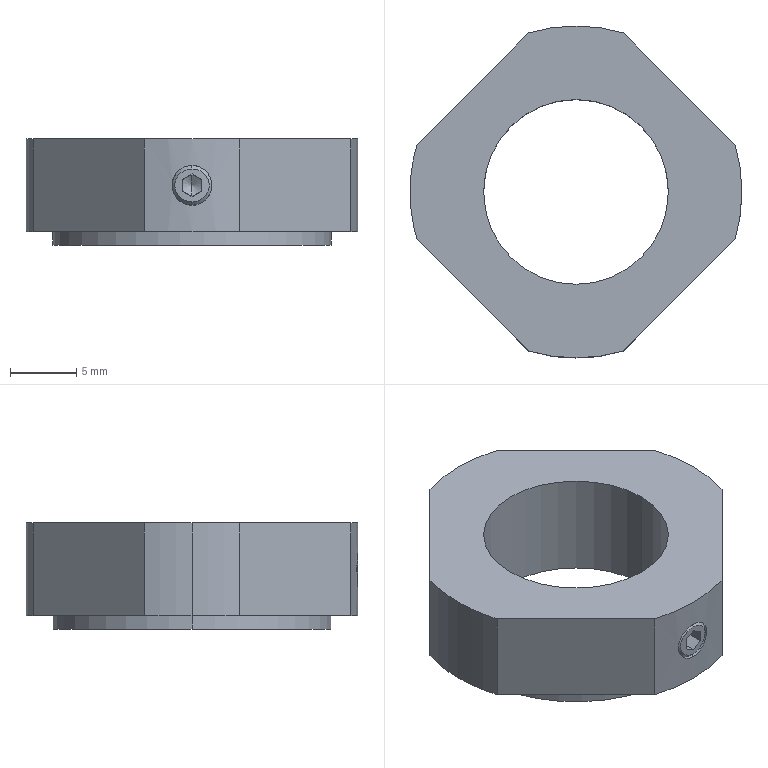Part | SolidWorks | features BaseBody 1 | 1 solid | 40 faces | box 25 x 25 x 8 mm | volume 2221 mm3 | plane 20 | cylinder 14 | cone 6 | commonest cylinder face diameters 25 x6 3 x4 13.917 x2 21 x2
STEP:
#1=CARTESIAN_POINT('',(-127.496,1824.586,28.5));
#2=VERTEX_POINT('',#1);
#3=CARTESIAN_POINT('',(-127.496,1824.586,25.5));
#4=VERTEX_POINT('',#3);
#5=CARTESIAN_POINT('',(-127.496,1824.586,28.5));
#6=CARTESIAN_POINT('',(-127.398,1824.586,28.5));
#7=CARTESIAN_POINT('',(-127.298,1824.588,28.49));
#8=CARTESIAN_POINT('',(-127.105,1824.596,28.452));
#9=CARTESIAN_POINT('',(-127.012,1824.602,28.423));
#10=CARTESIAN_POINT('',(-126.739,1824.624,28.31));
#11=CARTESIAN_POINT('',(-126.574,1824.645,28.2));
#12=CARTESIAN_POINT('',(-126.365,1824.678,27.991));
#13=CARTESIAN_POINT('',(-126.303,1824.688,27.915));
#14=CARTESIAN_POINT('',(-126.195,1824.708,27.753));
#15=CARTESIAN_POINT('',(-126.148,1824.717,27.665));
#16=CARTESIAN_POINT('',(-126.035,1824.74,27.393));
#17=CARTESIAN_POINT('',(-125.996,1824.749,27.197));
#18=CARTESIAN_POINT('',(-125.996,1824.749,26.899));
#19=CARTESIAN_POINT('',(-126.006,1824.747,26.802));
#20=CARTESIAN_POINT('',(-126.044,1824.739,26.61));
#21=CARTESIAN_POINT('',(-126.073,1824.732,26.514));
#22=CARTESIAN_POINT('',(-126.149,1824.717,26.333));
#23=CARTESIAN_POINT('',(-126.195,1824.708,26.247));
#24=CARTESIAN_POINT('',(-126.304,1824.688,26.084));
#25=CARTESIAN_POINT('',(-126.367,1824.677,26.007));
#26=CARTESIAN_POINT('',(-126.574,1824.645,25.801));
#27=CARTESIAN_POINT('',(-126.741,1824.624,25.689));
#28=CARTESIAN_POINT('',(-127.102,1824.594,25.54));
#29=CARTESIAN_POINT('',(-127.3,1824.586,25.5));
#30=CARTESIAN_POINT('',(-127.496,1824.586,25.5));
#31=B_SPLINE_CURVE_WITH_KNOTS('',3,(#5,#6,#7,#8,#9,#10,#11,#12,#13,#14,#15,#16,#17,#18,#19,#20,#21,#22,#23,#24,#25,#26,#27,#28,#29,#30),.UNSPECIFIED.,.F.,.F.,(4,2,2,2,2,2,2,2,2,2,2,2,4),(0.007054,0.007348,0.007642,0.00823,0.008524,0.008818,0.009406,0.009699,0.009993,0.01029,0.01058,0.01117,0.01176),.UNSPECIFIED.);
#32=EDGE_CURVE('',#2,#4,#31,.T.);
#33=ORIENTED_EDGE('',*,*,#32,.F.);
#34=CARTESIAN_POINT('',(-127.496,1824.586,25.5));
#35=CARTESIAN_POINT('',(-127.594,1824.586,25.5));
#36=CARTESIAN_POINT('',(-127.694,1824.588,25.51));
#37=CARTESIAN_POINT('',(-127.886,1824.596,25.548));
#38=CARTESIAN_POINT('',(-127.98,1824.602,25.577));
#39=CARTESIAN_POINT('',(-128.253,1824.624,25.69));
#40=CARTESIAN_POINT('',(-128.418,1824.645,25.8));
#41=CARTESIAN_POINT('',(-128.626,1824.678,26.009));
#42=CARTESIAN_POINT('',(-128.688,1824.688,26.085));
#43=CARTESIAN_POINT('',(-128.797,1824.708,26.247));
#44=CARTESIAN_POINT('',(-128.844,1824.717,26.335));
#45=CARTESIAN_POINT('',(-128.957,1824.74,26.607));
#46=CARTESIAN_POINT('',(-128.996,1824.749,26.802));
#47=CARTESIAN_POINT('',(-128.996,1824.749,27.101));
#48=CARTESIAN_POINT('',(-128.986,1824.747,27.198));
#49=CARTESIAN_POINT('',(-128.947,1824.739,27.39));
#50=CARTESIAN_POINT('',(-128.918,1824.732,27.486));
#51=CARTESIAN_POINT('',(-128.843,1824.717,27.667));
#52=CARTESIAN_POINT('',(-128.797,1824.708,27.753));
#53=CARTESIAN_POINT('',(-128.688,1824.688,27.916));
#54=CARTESIAN_POINT('',(-128.625,1824.677,27.993));
#55=CARTESIAN_POINT('',(-128.418,1824.645,28.199));
#56=CARTESIAN_POINT('',(-128.251,1824.624,28.311));
#57=CARTESIAN_POINT('',(-127.89,1824.594,28.46));
#58=CARTESIAN_POINT('',(-127.692,1824.586,28.5));
#59=CARTESIAN_POINT('',(-127.496,1824.586,28.5));
#60=B_SPLINE_CURVE_WITH_KNOTS('',3,(#34,#35,#36,#37,#38,#39,#40,#41,#42,#43,#44,#45,#46,#47,#48,#49,#50,#51,#52,#53,#54,#55,#56,#57,#58,#59),.UNSPECIFIED.,.F.,.F.,(4,2,2,2,2,2,2,2,2,2,2,2,4),(0.002352,0.002646,0.00294,0.003528,0.003822,0.004116,0.004703,0.004997,0.005291,0.005585,0.005879,0.006467,0.007054),.UNSPECIFIED.);
#61=EDGE_CURVE('',#4,#2,#60,.T.);
#62=ORIENTED_EDGE('',*,*,#61,.F.);
#63=EDGE_LOOP('',(#33,#62));
#64=FACE_BOUND('',#63,.T.);
#65=CARTESIAN_POINT('',(-120.537,1831.544,30.5));
#66=VERTEX_POINT('',#65);
#67=CARTESIAN_POINT('',(-134.454,1831.544,30.5));
#68=VERTEX_POINT('',#67);
#69=CARTESIAN_POINT('',(-127.496,1831.544,30.5));
#70=DIRECTION('',(0.,0.,-1.));
#71=DIRECTION('',(-1.,0.,0.));
#72=AXIS2_PLACEMENT_3D('',#69,#70,#71);
#73=CIRCLE('',#72,6.959);
#74=EDGE_CURVE('',#66,#68,#73,.T.);
#75=ORIENTED_EDGE('',*,*,#74,.F.);
#76=CARTESIAN_POINT('',(-120.537,1831.544,22.5));
#77=VERTEX_POINT('',#76);
#78=CARTESIAN_POINT('',(-120.537,1831.544,22.5));
#79=DIRECTION('',(0.,0.,-1.));
#80=VECTOR('',#79,1000.);
#81=LINE('',#78,#80);
#82=EDGE_CURVE('',#66,#77,#81,.T.);
#83=ORIENTED_EDGE('',*,*,#82,.T.);
#84=CARTESIAN_POINT('',(-134.454,1831.544,22.5));
#85=VERTEX_POINT('',#84);
#86=CARTESIAN_POINT('',(-127.496,1831.544,22.5));
#87=DIRECTION('',(0.,0.,1.));
#88=DIRECTION('',(-1.,0.,0.));
#89=AXIS2_PLACEMENT_3D('',#86,#87,#88);
#90=CIRCLE('',#89,6.959);
#91=EDGE_CURVE('',#85,#77,#90,.T.);
#92=ORIENTED_EDGE('',*,*,#91,.F.);
#93=CARTESIAN_POINT('',(-134.454,1831.544,22.5));
#94=DIRECTION('',(0.,0.,-1.));
#95=VECTOR('',#94,1000.);
#96=LINE('',#93,#95);
#97=EDGE_CURVE('',#68,#85,#96,.T.);
#98=ORIENTED_EDGE('',*,*,#97,.F.);
#99=EDGE_LOOP('',(#75,#83,#92,#98));
#100=FACE_OUTER_BOUND('',#99,.T.);
#101=CARTESIAN_POINT('',(-127.496,1831.544,22.5));
#102=DIRECTION('',(0.,0.,-1.));
#103=DIRECTION('',(-1.,0.,0.));
#104=AXIS2_PLACEMENT_3D('',#101,#102,#103);
#105=CYLINDRICAL_SURFACE('',#104,6.959);
#106=ADVANCED_FACE('',(#64,#100),#105,.F.);
#107=CARTESIAN_POINT('',(-139.996,1831.544,30.5));
#108=VERTEX_POINT('',#107);
#109=CARTESIAN_POINT('',(-139.472,1827.964,30.5));
#110=VERTEX_POINT('',#109);
#111=CARTESIAN_POINT('',(-127.496,1831.544,30.5));
#112=DIRECTION('',(0.,0.,1.));
#113=DIRECTION('',(-1.,0.,0.));
#114=AXIS2_PLACEMENT_3D('',#111,#112,#113);
#115=CIRCLE('',#114,12.5);
#116=EDGE_CURVE('',#108,#110,#115,.T.);
#117=ORIENTED_EDGE('',*,*,#116,.F.);
#118=CARTESIAN_POINT('',(-139.996,1831.544,23.5));
#119=VERTEX_POINT('',#118);
#120=CARTESIAN_POINT('',(-139.996,1831.544,22.5));
#121=DIRECTION('',(0.,0.,-1.));
#122=VECTOR('',#121,1000.);
#123=LINE('',#120,#122);
#124=EDGE_CURVE('',#108,#119,#123,.T.);
#125=ORIENTED_EDGE('',*,*,#124,.T.);
#126=CARTESIAN_POINT('',(-139.472,1827.964,23.5));
#127=VERTEX_POINT('',#126);
#128=CARTESIAN_POINT('',(-127.496,1831.544,23.5));
#129=DIRECTION('',(0.,0.,1.));
#130=DIRECTION('',(-1.,0.,0.));
#131=AXIS2_PLACEMENT_3D('',#128,#129,#130);
#132=CIRCLE('',#131,12.5);
#133=EDGE_CURVE('',#119,#127,#132,.T.);
#134=ORIENTED_EDGE('',*,*,#133,.T.);
#135=CARTESIAN_POINT('',(-139.472,1827.964,30.5));
#136=DIRECTION('',(0.,0.,-1.));
#137=VECTOR('',#136,1000.);
#138=LINE('',#135,#137);
#139=EDGE_CURVE('',#110,#127,#138,.T.);
#140=ORIENTED_EDGE('',*,*,#139,.F.);
#141=EDGE_LOOP('',(#117,#125,#134,#140));
#142=FACE_OUTER_BOUND('',#141,.T.);
#143=CARTESIAN_POINT('',(-127.496,1831.544,22.5));
#144=DIRECTION('',(0.,0.,-1.));
#145=DIRECTION('',(-1.,0.,0.));
#146=AXIS2_PLACEMENT_3D('',#143,#144,#145);
#147=CYLINDRICAL_SURFACE('',#146,12.5);
#148=ADVANCED_FACE('',(#142),#147,.T.);
#149=CARTESIAN_POINT('',(-127.496,1823.544,25.5));
#150=VERTEX_POINT('',#149);
#151=CARTESIAN_POINT('',(-127.496,1823.544,28.5));
#152=VERTEX_POINT('',#151);
#153=CARTESIAN_POINT('',(-127.496,1823.544,27.));
#154=DIRECTION('',(0.,1.,0.));
#155=DIRECTION('',(0.,0.,1.));
#156=AXIS2_PLACEMENT_3D('',#153,#154,#155);
#157=CIRCLE('',#156,1.5);
#158=EDGE_CURVE('',#150,#152,#157,.T.);
#159=ORIENTED_EDGE('',*,*,#158,.F.);
#160=CARTESIAN_POINT('',(-127.496,1820.695,25.5));
#161=DIRECTION('',(0.,1.,0.));
#162=VECTOR('',#161,1000.);
#163=LINE('',#160,#162);
#164=EDGE_CURVE('',#150,#4,#163,.T.);
#165=ORIENTED_EDGE('',*,*,#164,.T.);
#166=ORIENTED_EDGE('',*,*,#61,.T.);
#167=CARTESIAN_POINT('',(-127.496,1820.695,28.5));
#168=DIRECTION('',(0.,1.,0.));
#169=VECTOR('',#168,1000.);
#170=LINE('',#167,#169);
#171=EDGE_CURVE('',#152,#2,#170,.T.);
#172=ORIENTED_EDGE('',*,*,#171,.F.);
#173=EDGE_LOOP('',(#159,#165,#166,#172));
#174=FACE_OUTER_BOUND('',#173,.T.);
#175=CARTESIAN_POINT('',(-127.496,1820.695,27.));
#176=DIRECTION('',(0.,1.,0.));
#177=DIRECTION('',(0.,0.,1.));
#178=AXIS2_PLACEMENT_3D('',#175,#176,#177);
#179=CYLINDRICAL_SURFACE('',#178,1.5);
#180=ADVANCED_FACE('',(#174),#179,.F.);
#181=CARTESIAN_POINT('',(-127.496,1819.044,25.5));
#182=VERTEX_POINT('',#181);
#183=CARTESIAN_POINT('',(-127.496,1819.044,28.5));
#184=VERTEX_POINT('',#183);
#185=CARTESIAN_POINT('',(-127.496,1819.044,25.5));
#186=CARTESIAN_POINT('',(-127.595,1819.044,25.5));
#187=CARTESIAN_POINT('',(-127.692,1819.045,25.51));
#188=CARTESIAN_POINT('',(-127.884,1819.05,25.548));
#189=CARTESIAN_POINT('',(-127.979,1819.053,25.577));
#190=CARTESIAN_POINT('',(-128.161,1819.061,25.652));
#191=CARTESIAN_POINT('',(-128.247,1819.066,25.698));
#192=CARTESIAN_POINT('',(-128.41,1819.077,25.807));
#193=CARTESIAN_POINT('',(-128.487,1819.083,25.87));
#194=CARTESIAN_POINT('',(-128.694,1819.101,26.077));
#195=CARTESIAN_POINT('',(-128.806,1819.113,26.244));
#196=CARTESIAN_POINT('',(-128.956,1819.129,26.605));
#197=CARTESIAN_POINT('',(-128.996,1819.134,26.802));
#198=CARTESIAN_POINT('',(-128.996,1819.134,27.099));
#199=CARTESIAN_POINT('',(-128.986,1819.133,27.197));
#200=CARTESIAN_POINT('',(-128.948,1819.129,27.388));
#201=CARTESIAN_POINT('',(-128.919,1819.125,27.484));
#202=CARTESIAN_POINT('',(-128.844,1819.117,27.665));
#203=CARTESIAN_POINT('',(-128.798,1819.112,27.751));
#204=CARTESIAN_POINT('',(-128.689,1819.101,27.914));
#205=CARTESIAN_POINT('',(-128.626,1819.095,27.991));
#206=CARTESIAN_POINT('',(-128.419,1819.077,28.199));
#207=CARTESIAN_POINT('',(-128.252,1819.066,28.31));
#208=CARTESIAN_POINT('',(-127.891,1819.049,28.46));
#209=CARTESIAN_POINT('',(-127.694,1819.044,28.5));
#210=CARTESIAN_POINT('',(-127.496,1819.044,28.5));
#211=B_SPLINE_CURVE_WITH_KNOTS('',3,(#185,#186,#187,#188,#189,#190,#191,#192,#193,#194,#195,#196,#197,#198,#199,#200,#201,#202,#203,#204,#205,#206,#207,#208,#209,#210),.UNSPECIFIED.,.F.,.F.,(4,2,2,2,2,2,2,2,2,2,2,2,4),(-0.004691,-0.004397,-0.004104,-0.003811,-0.003518,-0.002932,-0.002345,-0.002052,-0.001759,-0.001466,-0.001173,-0.0005863,0.),.UNSPECIFIED.);
#212=EDGE_CURVE('',#182,#184,#211,.T.);
#213=ORIENTED_EDGE('',*,*,#212,.F.);
#214=CARTESIAN_POINT('',(-127.496,1819.315,25.5));
#215=VERTEX_POINT('',#214);
#216=CARTESIAN_POINT('',(-127.496,1820.695,25.5));
#217=DIRECTION('',(0.,1.,0.));
#218=VECTOR('',#217,1000.);
#219=LINE('',#216,#218);
#220=EDGE_CURVE('',#182,#215,#219,.T.);
#221=ORIENTED_EDGE('',*,*,#220,.T.);
#222=CARTESIAN_POINT('',(-127.496,1819.315,28.5));
#223=VERTEX_POINT('',#222);
#224=CARTESIAN_POINT('',(-127.496,1819.315,27.));
#225=DIRECTION('',(0.,-1.,0.));
#226=DIRECTION('',(0.,0.,1.));
#227=AXIS2_PLACEMENT_3D('',#224,#225,#226);
#228=CIRCLE('',#227,1.5);
#229=EDGE_CURVE('',#223,#215,#228,.T.);
#230=ORIENTED_EDGE('',*,*,#229,.F.);
#231=CARTESIAN_POINT('',(-127.496,1820.695,28.5));
#232=DIRECTION('',(0.,1.,0.));
#233=VECTOR('',#232,1000.);
#234=LINE('',#231,#233);
#235=EDGE_CURVE('',#184,#223,#234,.T.);
#236=ORIENTED_EDGE('',*,*,#235,.F.);
#237=EDGE_LOOP('',(#213,#221,#230,#236));
#238=FACE_OUTER_BOUND('',#237,.T.);
#239=CARTESIAN_POINT('',(-127.496,1820.695,27.));
#240=DIRECTION('',(0.,1.,0.));
#241=DIRECTION('',(0.,0.,1.));
#242=AXIS2_PLACEMENT_3D('',#239,#240,#241);
#243=CYLINDRICAL_SURFACE('',#242,1.5);
#244=ADVANCED_FACE('',(#238),#243,.F.);
#245=CARTESIAN_POINT('',(-127.496,1824.044,26.));
#246=VERTEX_POINT('',#245);
#247=CARTESIAN_POINT('',(-127.496,1824.044,28.));
#248=VERTEX_POINT('',#247);
#249=CARTESIAN_POINT('',(-127.496,1824.044,27.));
#250=DIRECTION('',(0.,-1.,0.));
#251=DIRECTION('',(0.,0.,-1.));
#252=AXIS2_PLACEMENT_3D('',#249,#250,#251);
#253=CIRCLE('',#252,1.);
#254=EDGE_CURVE('',#246,#248,#253,.T.);
#255=ORIENTED_EDGE('',*,*,#254,.T.);
#256=CARTESIAN_POINT('',(-127.496,1823.544,28.5));
#257=DIRECTION('',(0.,-0.7071,0.7071));
#258=VECTOR('',#257,1000.);
#259=LINE('',#256,#258);
#260=EDGE_CURVE('',#248,#152,#259,.T.);
#261=ORIENTED_EDGE('',*,*,#260,.T.);
#262=CARTESIAN_POINT('',(-127.496,1823.544,27.));
#263=DIRECTION('',(0.,1.,0.));
#264=DIRECTION('',(0.,0.,1.));
#265=AXIS2_PLACEMENT_3D('',#262,#263,#264);
#266=CIRCLE('',#265,1.5);
#267=EDGE_CURVE('',#152,#150,#266,.T.);
#268=ORIENTED_EDGE('',*,*,#267,.T.);
#269=CARTESIAN_POINT('',(-127.496,1823.544,25.5));
#270=DIRECTION('',(0.,-0.7071,-0.7071));
#271=VECTOR('',#270,1000.);
#272=LINE('',#269,#271);
#273=EDGE_CURVE('',#246,#150,#272,.T.);
#274=ORIENTED_EDGE('',*,*,#273,.F.);
#275=EDGE_LOOP('',(#255,#261,#268,#274));
#276=FACE_OUTER_BOUND('',#275,.T.);
#277=CARTESIAN_POINT('',(-127.496,1823.544,27.));
#278=DIRECTION('',(0.,-1.,0.));
#279=DIRECTION('',(0.,0.,-1.));
#280=AXIS2_PLACEMENT_3D('',#277,#278,#279);
#281=CONICAL_SURFACE('',#280,1.5,0.7854);
#282=ADVANCED_FACE('',(#276),#281,.T.);
#283=CARTESIAN_POINT('',(-116.996,1831.544,23.5));
#284=VERTEX_POINT('',#283);
#285=CARTESIAN_POINT('',(-137.996,1831.544,23.5));
#286=VERTEX_POINT('',#285);
#287=CARTESIAN_POINT('',(-127.496,1831.544,23.5));
#288=DIRECTION('',(0.,0.,1.));
#289=DIRECTION('',(-1.,0.,0.));
#290=AXIS2_PLACEMENT_3D('',#287,#288,#289);
#291=CIRCLE('',#290,10.5);
#292=EDGE_CURVE('',#284,#286,#291,.T.);
#293=ORIENTED_EDGE('',*,*,#292,.F.);
#294=CARTESIAN_POINT('',(-116.996,1831.544,22.5));
#295=VERTEX_POINT('',#294);
#296=CARTESIAN_POINT('',(-116.996,1831.544,22.5));
#297=DIRECTION('',(0.,0.,-1.));
#298=VECTOR('',#297,1000.);
#299=LINE('',#296,#298);
#300=EDGE_CURVE('',#284,#295,#299,.T.);
#301=ORIENTED_EDGE('',*,*,#300,.T.);
#302=CARTESIAN_POINT('',(-137.996,1831.544,22.5));
#303=VERTEX_POINT('',#302);
#304=CARTESIAN_POINT('',(-127.496,1831.544,22.5));
#305=DIRECTION('',(0.,0.,-1.));
#306=DIRECTION('',(-1.,0.,0.));
#307=AXIS2_PLACEMENT_3D('',#304,#305,#306);
#308=CIRCLE('',#307,10.5);
#309=EDGE_CURVE('',#303,#295,#308,.T.);
#310=ORIENTED_EDGE('',*,*,#309,.F.);
#311=CARTESIAN_POINT('',(-137.996,1831.544,22.5));
#312=DIRECTION('',(0.,0.,-1.));
#313=VECTOR('',#312,1000.);
#314=LINE('',#311,#313);
#315=EDGE_CURVE('',#286,#303,#314,.T.);
#316=ORIENTED_EDGE('',*,*,#315,.F.);
#317=EDGE_LOOP('',(#293,#301,#310,#316));
#318=FACE_OUTER_BOUND('',#317,.T.);
#319=CARTESIAN_POINT('',(-127.496,1831.544,22.5));
#320=DIRECTION('',(0.,0.,-1.));
#321=DIRECTION('',(-1.,0.,0.));
#322=AXIS2_PLACEMENT_3D('',#319,#320,#321);
#323=CYLINDRICAL_SURFACE('',#322,10.5);
#324=ADVANCED_FACE('',(#318),#323,.T.);
#325=CARTESIAN_POINT('',(-127.496,1819.044,28.23));
#326=VERTEX_POINT('',#325);
#327=CARTESIAN_POINT('',(-127.496,1819.044,25.77));
#328=VERTEX_POINT('',#327);
#329=CARTESIAN_POINT('',(-127.496,1819.044,28.23));
#330=CARTESIAN_POINT('',(-127.329,1819.044,28.23));
#331=CARTESIAN_POINT('',(-127.166,1819.047,28.199));
#332=CARTESIAN_POINT('',(-126.856,1819.059,28.081));
#333=CARTESIAN_POINT('',(-126.715,1819.068,27.994));
#334=CARTESIAN_POINT('',(-126.47,1819.086,27.768));
#335=CARTESIAN_POINT('',(-126.371,1819.095,27.632));
#336=CARTESIAN_POINT('',(-126.235,1819.108,27.332));
#337=CARTESIAN_POINT('',(-126.199,1819.111,27.167));
#338=CARTESIAN_POINT('',(-126.199,1819.111,26.917));
#339=CARTESIAN_POINT('',(-126.208,1819.111,26.835));
#340=CARTESIAN_POINT('',(-126.243,1819.107,26.673));
#341=CARTESIAN_POINT('',(-126.269,1819.104,26.594));
#342=CARTESIAN_POINT('',(-126.371,1819.095,26.368));
#343=CARTESIAN_POINT('',(-126.47,1819.086,26.231));
#344=CARTESIAN_POINT('',(-126.712,1819.068,26.008));
#345=CARTESIAN_POINT('',(-126.856,1819.059,25.919));
#346=CARTESIAN_POINT('',(-127.164,1819.047,25.801));
#347=CARTESIAN_POINT('',(-127.329,1819.044,25.77));
#348=CARTESIAN_POINT('',(-127.496,1819.044,25.77));
#349=B_SPLINE_CURVE_WITH_KNOTS('',3,(#329,#330,#331,#332,#333,#334,#335,#336,#337,#338,#339,#340,#341,#342,#343,#344,#345,#346,#347,#348),.UNSPECIFIED.,.F.,.F.,(4,2,2,2,2,2,2,2,2,4),(0.001976,0.00247,0.002964,0.003458,0.003952,0.004199,0.004446,0.00494,0.005434,0.005928),.UNSPECIFIED.);
#350=EDGE_CURVE('',#326,#328,#349,.T.);
#351=ORIENTED_EDGE('',*,*,#350,.T.);
#352=CARTESIAN_POINT('',(-127.496,1819.315,25.5));
#353=DIRECTION('',(0.,0.7071,-0.7071));
#354=VECTOR('',#353,1000.);
#355=LINE('',#352,#354);
#356=EDGE_CURVE('',#328,#215,#355,.T.);
#357=ORIENTED_EDGE('',*,*,#356,.T.);
#358=CARTESIAN_POINT('',(-127.496,1819.315,27.));
#359=DIRECTION('',(0.,-1.,0.));
#360=DIRECTION('',(0.,0.,1.));
#361=AXIS2_PLACEMENT_3D('',#358,#359,#360);
#362=CIRCLE('',#361,1.5);
#363=EDGE_CURVE('',#215,#223,#362,.T.);
#364=ORIENTED_EDGE('',*,*,#363,.T.);
#365=CARTESIAN_POINT('',(-127.496,1819.315,28.5));
#366=DIRECTION('',(0.,0.7071,0.7071));
#367=VECTOR('',#366,1000.);
#368=LINE('',#365,#367);
#369=EDGE_CURVE('',#326,#223,#368,.T.);
#370=ORIENTED_EDGE('',*,*,#369,.F.);
#371=EDGE_LOOP('',(#351,#357,#364,#370));
#372=FACE_OUTER_BOUND('',#371,.T.);
#373=CARTESIAN_POINT('',(-127.496,1819.315,27.));
#374=DIRECTION('',(0.,1.,0.));
#375=DIRECTION('',(0.,0.,1.));
#376=AXIS2_PLACEMENT_3D('',#373,#374,#375);
#377=CONICAL_SURFACE('',#376,1.5,0.7854);
#378=ADVANCED_FACE('',(#372),#377,.T.);
#379=CARTESIAN_POINT('',(-127.496,1820.695,27.));
#380=VERTEX_POINT('',#379);
#381=CARTESIAN_POINT('',(-127.496,1820.244,26.25));
#382=VERTEX_POINT('',#381);
#383=CARTESIAN_POINT('',(-127.496,1820.244,26.25));
#384=DIRECTION('',(0.,-0.515,-0.8572));
#385=VECTOR('',#384,1000.);
#386=LINE('',#383,#385);
#387=EDGE_CURVE('',#380,#382,#386,.T.);
#388=ORIENTED_EDGE('',*,*,#387,.F.);
#389=CARTESIAN_POINT('',(-127.496,1820.244,27.75));
#390=VERTEX_POINT('',#389);
#391=CARTESIAN_POINT('',(-127.496,1820.244,27.75));
#392=DIRECTION('',(0.,-0.515,0.8572));
#393=VECTOR('',#392,1000.);
#394=LINE('',#391,#393);
#395=EDGE_CURVE('',#380,#390,#394,.T.);
#396=ORIENTED_EDGE('',*,*,#395,.T.);
#397=CARTESIAN_POINT('',(-127.871,1820.244,27.65));
#398=VERTEX_POINT('',#397);
#399=CARTESIAN_POINT('',(-127.496,1820.244,27.));
#400=DIRECTION('',(0.,1.,0.));
#401=DIRECTION('',(0.,0.,-1.));
#402=AXIS2_PLACEMENT_3D('',#399,#400,#401);
#403=CIRCLE('',#402,0.75);
#404=EDGE_CURVE('',#398,#390,#403,.T.);
#405=ORIENTED_EDGE('',*,*,#404,.F.);
#406=CARTESIAN_POINT('',(-128.246,1820.244,27.));
#407=VERTEX_POINT('',#406);
#408=CARTESIAN_POINT('',(-127.496,1820.244,27.));
#409=DIRECTION('',(0.,1.,0.));
#410=DIRECTION('',(0.,0.,-1.));
#411=AXIS2_PLACEMENT_3D('',#408,#409,#410);
#412=CIRCLE('',#411,0.75);
#413=EDGE_CURVE('',#407,#398,#412,.T.);
#414=ORIENTED_EDGE('',*,*,#413,.F.);
#415=CARTESIAN_POINT('',(-127.871,1820.244,26.35));
#416=VERTEX_POINT('',#415);
#417=CARTESIAN_POINT('',(-127.496,1820.244,27.));
#418=DIRECTION('',(0.,1.,0.));
#419=DIRECTION('',(0.,0.,-1.));
#420=AXIS2_PLACEMENT_3D('',#417,#418,#419);
#421=CIRCLE('',#420,0.75);
#422=EDGE_CURVE('',#416,#407,#421,.T.);
#423=ORIENTED_EDGE('',*,*,#422,.F.);
#424=CARTESIAN_POINT('',(-127.496,1820.244,27.));
#425=DIRECTION('',(0.,1.,0.));
#426=DIRECTION('',(0.,0.,-1.));
#427=AXIS2_PLACEMENT_3D('',#424,#425,#426);
#428=CIRCLE('',#427,0.75);
#429=EDGE_CURVE('',#382,#416,#428,.T.);
#430=ORIENTED_EDGE('',*,*,#429,.F.);
#431=EDGE_LOOP('',(#388,#396,#405,#414,#423,#430));
#432=FACE_OUTER_BOUND('',#431,.T.);
#433=CARTESIAN_POINT('',(-127.496,1820.244,27.));
#434=DIRECTION('',(0.,-1.,0.));
#435=DIRECTION('',(0.,0.,-1.));
#436=AXIS2_PLACEMENT_3D('',#433,#434,#435);
#437=CONICAL_SURFACE('',#436,0.75,1.03);
#438=ADVANCED_FACE('',(#432),#437,.F.);
#439=CARTESIAN_POINT('',(-127.496,1831.544,30.5));
#440=DIRECTION('',(0.,0.,-1.));
#441=DIRECTION('',(-1.,0.,0.));
#442=AXIS2_PLACEMENT_3D('',#439,#440,#441);
#443=CIRCLE('',#442,6.959);
#444=EDGE_CURVE('',#68,#66,#443,.T.);
#445=ORIENTED_EDGE('',*,*,#444,.T.);
#446=ORIENTED_EDGE('',*,*,#74,.T.);
#447=EDGE_LOOP('',(#445,#446));
#448=FACE_BOUND('',#447,.T.);
#449=CARTESIAN_POINT('',(-123.916,1819.568,30.5));
#450=VERTEX_POINT('',#449);
#451=CARTESIAN_POINT('',(-115.519,1827.964,30.5));
#452=VERTEX_POINT('',#451);
#453=CARTESIAN_POINT('',(-123.916,1819.568,30.5));
#454=DIRECTION('',(0.7071,0.7071,0.));
#455=VECTOR('',#454,1000.);
#456=LINE('',#453,#455);
#457=EDGE_CURVE('',#450,#452,#456,.T.);
#458=ORIENTED_EDGE('',*,*,#457,.T.);
#459=CARTESIAN_POINT('',(-115.519,1835.124,30.5));
#460=VERTEX_POINT('',#459);
#461=CARTESIAN_POINT('',(-127.496,1831.544,30.5));
#462=DIRECTION('',(0.,0.,1.));
#463=DIRECTION('',(-1.,0.,0.));
#464=AXIS2_PLACEMENT_3D('',#461,#462,#463);
#465=CIRCLE('',#464,12.5);
#466=EDGE_CURVE('',#452,#460,#465,.T.);
#467=ORIENTED_EDGE('',*,*,#466,.T.);
#468=CARTESIAN_POINT('',(-123.916,1843.52,30.5));
#469=VERTEX_POINT('',#468);
#470=CARTESIAN_POINT('',(-115.519,1835.124,30.5));
#471=DIRECTION('',(-0.7071,0.7071,0.));
#472=VECTOR('',#471,1000.);
#473=LINE('',#470,#472);
#474=EDGE_CURVE('',#460,#469,#473,.T.);
#475=ORIENTED_EDGE('',*,*,#474,.T.);
#476=CARTESIAN_POINT('',(-131.076,1843.52,30.5));
#477=VERTEX_POINT('',#476);
#478=CARTESIAN_POINT('',(-127.496,1831.544,30.5));
#479=DIRECTION('',(0.,0.,1.));
#480=DIRECTION('',(-1.,0.,0.));
#481=AXIS2_PLACEMENT_3D('',#478,#479,#480);
#482=CIRCLE('',#481,12.5);
#483=EDGE_CURVE('',#469,#477,#482,.T.);
#484=ORIENTED_EDGE('',*,*,#483,.T.);
#485=CARTESIAN_POINT('',(-139.472,1835.124,30.5));
#486=VERTEX_POINT('',#485);
#487=CARTESIAN_POINT('',(-131.076,1843.52,30.5));
#488=DIRECTION('',(-0.7071,-0.7071,0.));
#489=VECTOR('',#488,1000.);
#490=LINE('',#487,#489);
#491=EDGE_CURVE('',#477,#486,#490,.T.);
#492=ORIENTED_EDGE('',*,*,#491,.T.);
#493=CARTESIAN_POINT('',(-127.496,1831.544,30.5));
#494=DIRECTION('',(0.,0.,1.));
#495=DIRECTION('',(-1.,0.,0.));
#496=AXIS2_PLACEMENT_3D('',#493,#494,#495);
#497=CIRCLE('',#496,12.5);
#498=EDGE_CURVE('',#486,#108,#497,.T.);
#499=ORIENTED_EDGE('',*,*,#498,.T.);
#500=ORIENTED_EDGE('',*,*,#116,.T.);
#501=CARTESIAN_POINT('',(-131.076,1819.568,30.5));
#502=VERTEX_POINT('',#501);
#503=CARTESIAN_POINT('',(-139.472,1827.964,30.5));
#504=DIRECTION('',(0.7071,-0.7071,0.));
#505=VECTOR('',#504,1000.);
#506=LINE('',#503,#505);
#507=EDGE_CURVE('',#110,#502,#506,.T.);
#508=ORIENTED_EDGE('',*,*,#507,.T.);
#509=CARTESIAN_POINT('',(-127.496,1831.544,30.5));
#510=DIRECTION('',(0.,0.,1.));
#511=DIRECTION('',(-1.,0.,0.));
#512=AXIS2_PLACEMENT_3D('',#509,#510,#511);
#513=CIRCLE('',#512,12.5);
#514=EDGE_CURVE('',#502,#450,#513,.T.);
#515=ORIENTED_EDGE('',*,*,#514,.T.);
#516=EDGE_LOOP('',(#458,#467,#475,#484,#492,#499,#500,#508,#515));
#517=FACE_OUTER_BOUND('',#516,.T.);
#518=CARTESIAN_POINT('',(-127.496,1831.544,30.5));
#519=DIRECTION('',(0.,0.,1.));
#520=DIRECTION('',(1.,0.,0.));
#521=AXIS2_PLACEMENT_3D('',#518,#519,#520);
#522=PLANE('',#521);
#523=ADVANCED_FACE('',(#448,#517),#522,.T.);
#524=ORIENTED_EDGE('',*,*,#82,.F.);
#525=ORIENTED_EDGE('',*,*,#444,.F.);
#526=ORIENTED_EDGE('',*,*,#97,.T.);
#527=CARTESIAN_POINT('',(-127.496,1831.544,22.5));
#528=DIRECTION('',(0.,0.,1.));
#529=DIRECTION('',(-1.,0.,0.));
#530=AXIS2_PLACEMENT_3D('',#527,#528,#529);
#531=CIRCLE('',#530,6.959);
#532=EDGE_CURVE('',#77,#85,#531,.T.);
#533=ORIENTED_EDGE('',*,*,#532,.F.);
#534=EDGE_LOOP('',(#524,#525,#526,#533));
#535=FACE_OUTER_BOUND('',#534,.T.);
#536=CARTESIAN_POINT('',(-127.496,1831.544,22.5));
#537=DIRECTION('',(0.,0.,-1.));
#538=DIRECTION('',(-1.,0.,0.));
#539=AXIS2_PLACEMENT_3D('',#536,#537,#538);
#540=CYLINDRICAL_SURFACE('',#539,6.959);
#541=ADVANCED_FACE('',(#535),#540,.F.);
#542=CARTESIAN_POINT('',(-115.519,1827.964,23.5));
#543=VERTEX_POINT('',#542);
#544=CARTESIAN_POINT('',(-115.519,1827.964,22.5));
#545=DIRECTION('',(0.,0.,-1.));
#546=VECTOR('',#545,1000.);
#547=LINE('',#544,#546);
#548=EDGE_CURVE('',#452,#543,#547,.T.);
#549=ORIENTED_EDGE('',*,*,#548,.T.);
#550=CARTESIAN_POINT('',(-115.519,1835.124,23.5));
#551=VERTEX_POINT('',#550);
#552=CARTESIAN_POINT('',(-127.496,1831.544,23.5));
#553=DIRECTION('',(0.,0.,1.));
#554=DIRECTION('',(-1.,0.,0.));
#555=AXIS2_PLACEMENT_3D('',#552,#553,#554);
#556=CIRCLE('',#555,12.5);
#557=EDGE_CURVE('',#543,#551,#556,.T.);
#558=ORIENTED_EDGE('',*,*,#557,.T.);
#559=CARTESIAN_POINT('',(-115.519,1835.124,22.5));
#560=DIRECTION('',(0.,0.,1.));
#561=VECTOR('',#560,1000.);
#562=LINE('',#559,#561);
#563=EDGE_CURVE('',#551,#460,#562,.T.);
#564=ORIENTED_EDGE('',*,*,#563,.T.);
#565=ORIENTED_EDGE('',*,*,#466,.F.);
#566=EDGE_LOOP('',(#549,#558,#564,#565));
#567=FACE_OUTER_BOUND('',#566,.T.);
#568=CARTESIAN_POINT('',(-127.496,1831.544,22.5));
#569=DIRECTION('',(0.,0.,-1.));
#570=DIRECTION('',(-1.,0.,0.));
#571=AXIS2_PLACEMENT_3D('',#568,#569,#570);
#572=CYLINDRICAL_SURFACE('',#571,12.5);
#573=ADVANCED_FACE('',(#567),#572,.T.);
#574=CARTESIAN_POINT('',(-123.916,1819.568,23.5));
#575=VERTEX_POINT('',#574);
#576=CARTESIAN_POINT('',(-123.916,1819.568,23.5));
#577=DIRECTION('',(0.7071,0.7071,0.));
#578=VECTOR('',#577,1000.);
#579=LINE('',#576,#578);
#580=EDGE_CURVE('',#575,#543,#579,.T.);
#581=ORIENTED_EDGE('',*,*,#580,.T.);
#582=ORIENTED_EDGE('',*,*,#548,.F.);
#583=ORIENTED_EDGE('',*,*,#457,.F.);
#584=CARTESIAN_POINT('',(-123.916,1819.568,30.5));
#585=DIRECTION('',(0.,0.,-1.));
#586=VECTOR('',#585,1000.);
#587=LINE('',#584,#586);
#588=EDGE_CURVE('',#450,#575,#587,.T.);
#589=ORIENTED_EDGE('',*,*,#588,.T.);
#590=EDGE_LOOP('',(#581,#582,#583,#589));
#591=FACE_OUTER_BOUND('',#590,.T.);
#592=CARTESIAN_POINT('',(-123.916,1819.568,30.5));
#593=DIRECTION('',(0.7071,-0.7071,0.));
#594=DIRECTION('',(0.7071,0.7071,0.));
#595=AXIS2_PLACEMENT_3D('',#592,#593,#594);
#596=PLANE('',#595);
#597=ADVANCED_FACE('',(#591),#596,.T.);
#598=CARTESIAN_POINT('',(-127.496,1819.044,28.5));
#599=CARTESIAN_POINT('',(-127.397,1819.044,28.5));
#600=CARTESIAN_POINT('',(-127.299,1819.045,28.49));
#601=CARTESIAN_POINT('',(-127.107,1819.05,28.452));
#602=CARTESIAN_POINT('',(-127.012,1819.053,28.423));
#603=CARTESIAN_POINT('',(-126.831,1819.061,28.348));
#604=CARTESIAN_POINT('',(-126.745,1819.066,28.302));
#605=CARTESIAN_POINT('',(-126.582,1819.077,28.193));
#606=CARTESIAN_POINT('',(-126.505,1819.083,28.13));
#607=CARTESIAN_POINT('',(-126.297,1819.101,27.923));
#608=CARTESIAN_POINT('',(-126.186,1819.113,27.756));
#609=CARTESIAN_POINT('',(-126.036,1819.129,27.395));
#610=CARTESIAN_POINT('',(-125.996,1819.134,27.198));
#611=CARTESIAN_POINT('',(-125.996,1819.134,26.901));
#612=CARTESIAN_POINT('',(-126.006,1819.133,26.803));
#613=CARTESIAN_POINT('',(-126.044,1819.129,26.612));
#614=CARTESIAN_POINT('',(-126.072,1819.125,26.516));
#615=CARTESIAN_POINT('',(-126.148,1819.117,26.335));
#616=CARTESIAN_POINT('',(-126.194,1819.112,26.249));
#617=CARTESIAN_POINT('',(-126.302,1819.101,26.086));
#618=CARTESIAN_POINT('',(-126.366,1819.095,26.009));
#619=CARTESIAN_POINT('',(-126.573,1819.077,25.801));
#620=CARTESIAN_POINT('',(-126.74,1819.066,25.69));
#621=CARTESIAN_POINT('',(-127.101,1819.049,25.54));
#622=CARTESIAN_POINT('',(-127.298,1819.044,25.5));
#623=CARTESIAN_POINT('',(-127.496,1819.044,25.5));
#624=B_SPLINE_CURVE_WITH_KNOTS('',3,(#598,#599,#600,#601,#602,#603,#604,#605,#606,#607,#608,#609,#610,#611,#612,#613,#614,#615,#616,#617,#618,#619,#620,#621,#622,#623),.UNSPECIFIED.,.F.,.F.,(4,2,2,2,2,2,2,2,2,2,2,2,4),(0.,0.0002932,0.0005863,0.0008795,0.001173,0.001759,0.002345,0.002639,0.002932,0.003225,0.003518,0.004104,0.004691),.UNSPECIFIED.);
#625=EDGE_CURVE('',#184,#182,#624,.T.);
#626=ORIENTED_EDGE('',*,*,#625,.T.);
#627=ORIENTED_EDGE('',*,*,#212,.T.);
#628=EDGE_LOOP('',(#626,#627));
#629=FACE_BOUND('',#628,.T.);
#630=ORIENTED_EDGE('',*,*,#588,.F.);
#631=ORIENTED_EDGE('',*,*,#514,.F.);
#632=CARTESIAN_POINT('',(-131.076,1819.568,23.5));
#633=VERTEX_POINT('',#632);
#634=CARTESIAN_POINT('',(-131.076,1819.568,22.5));
#635=DIRECTION('',(0.,0.,-1.));
#636=VECTOR('',#635,1000.);
#637=LINE('',#634,#636);
#638=EDGE_CURVE('',#502,#633,#637,.T.);
#639=ORIENTED_EDGE('',*,*,#638,.T.);
#640=CARTESIAN_POINT('',(-127.496,1831.544,23.5));
#641=DIRECTION('',(0.,0.,1.));
#642=DIRECTION('',(-1.,0.,0.));
#643=AXIS2_PLACEMENT_3D('',#640,#641,#642);
#644=CIRCLE('',#643,12.5);
#645=EDGE_CURVE('',#633,#575,#644,.T.);
#646=ORIENTED_EDGE('',*,*,#645,.T.);
#647=EDGE_LOOP('',(#630,#631,#639,#646));
#648=FACE_OUTER_BOUND('',#647,.T.);
#649=CARTESIAN_POINT('',(-127.496,1831.544,22.5));
#650=DIRECTION('',(0.,0.,-1.));
#651=DIRECTION('',(-1.,0.,0.));
#652=AXIS2_PLACEMENT_3D('',#649,#650,#651);
#653=CYLINDRICAL_SURFACE('',#652,12.5);
#654=ADVANCED_FACE('',(#629,#648),#653,.T.);
#655=CARTESIAN_POINT('',(-139.472,1827.964,23.5));
#656=DIRECTION('',(0.7071,-0.7071,0.));
#657=VECTOR('',#656,1000.);
#658=LINE('',#655,#657);
#659=EDGE_CURVE('',#127,#633,#658,.T.);
#660=ORIENTED_EDGE('',*,*,#659,.T.);
#661=ORIENTED_EDGE('',*,*,#638,.F.);
#662=ORIENTED_EDGE('',*,*,#507,.F.);
#663=ORIENTED_EDGE('',*,*,#139,.T.);
#664=EDGE_LOOP('',(#660,#661,#662,#663));
#665=FACE_OUTER_BOUND('',#664,.T.);
#666=CARTESIAN_POINT('',(-139.472,1827.964,30.5));
#667=DIRECTION('',(-0.7071,-0.7071,0.));
#668=DIRECTION('',(0.7071,-0.7071,0.));
#669=AXIS2_PLACEMENT_3D('',#666,#667,#668);
#670=PLANE('',#669);
#671=ADVANCED_FACE('',(#665),#670,.T.);
#672=ORIENTED_EDGE('',*,*,#124,.F.);
#673=ORIENTED_EDGE('',*,*,#498,.F.);
#674=CARTESIAN_POINT('',(-139.472,1835.124,23.5));
#675=VERTEX_POINT('',#674);
#676=CARTESIAN_POINT('',(-139.472,1835.124,22.5));
#677=DIRECTION('',(0.,0.,-1.));
#678=VECTOR('',#677,1000.);
#679=LINE('',#676,#678);
#680=EDGE_CURVE('',#486,#675,#679,.T.);
#681=ORIENTED_EDGE('',*,*,#680,.T.);
#682=CARTESIAN_POINT('',(-127.496,1831.544,23.5));
#683=DIRECTION('',(0.,0.,1.));
#684=DIRECTION('',(-1.,0.,0.));
#685=AXIS2_PLACEMENT_3D('',#682,#683,#684);
#686=CIRCLE('',#685,12.5);
#687=EDGE_CURVE('',#675,#119,#686,.T.);
#688=ORIENTED_EDGE('',*,*,#687,.T.);
#689=EDGE_LOOP('',(#672,#673,#681,#688));
#690=FACE_OUTER_BOUND('',#689,.T.);
#691=CARTESIAN_POINT('',(-127.496,1831.544,22.5));
#692=DIRECTION('',(0.,0.,-1.));
#693=DIRECTION('',(-1.,0.,0.));
#694=AXIS2_PLACEMENT_3D('',#691,#692,#693);
#695=CYLINDRICAL_SURFACE('',#694,12.5);
#696=ADVANCED_FACE('',(#690),#695,.T.);
#697=CARTESIAN_POINT('',(-131.076,1843.52,23.5));
#698=VERTEX_POINT('',#697);
#699=CARTESIAN_POINT('',(-139.472,1835.124,23.5));
#700=DIRECTION('',(-0.7071,-0.7071,0.));
#701=VECTOR('',#700,1000.);
#702=LINE('',#699,#701);
#703=EDGE_CURVE('',#698,#675,#702,.T.);
#704=ORIENTED_EDGE('',*,*,#703,.T.);
#705=ORIENTED_EDGE('',*,*,#680,.F.);
#706=ORIENTED_EDGE('',*,*,#491,.F.);
#707=CARTESIAN_POINT('',(-131.076,1843.52,30.5));
#708=DIRECTION('',(0.,0.,-1.));
#709=VECTOR('',#708,1000.);
#710=LINE('',#707,#709);
#711=EDGE_CURVE('',#477,#698,#710,.T.);
#712=ORIENTED_EDGE('',*,*,#711,.T.);
#713=EDGE_LOOP('',(#704,#705,#706,#712));
#714=FACE_OUTER_BOUND('',#713,.T.);
#715=CARTESIAN_POINT('',(-139.472,1835.124,30.5));
#716=DIRECTION('',(-0.7071,0.7071,0.));
#717=DIRECTION('',(-0.7071,-0.7071,0.));
#718=AXIS2_PLACEMENT_3D('',#715,#716,#717);
#719=PLANE('',#718);
#720=ADVANCED_FACE('',(#714),#719,.T.);
#721=ORIENTED_EDGE('',*,*,#711,.F.);
#722=ORIENTED_EDGE('',*,*,#483,.F.);
#723=CARTESIAN_POINT('',(-123.916,1843.52,23.5));
#724=VERTEX_POINT('',#723);
#725=CARTESIAN_POINT('',(-123.916,1843.52,22.5));
#726=DIRECTION('',(0.,0.,-1.));
#727=VECTOR('',#726,1000.);
#728=LINE('',#725,#727);
#729=EDGE_CURVE('',#469,#724,#728,.T.);
#730=ORIENTED_EDGE('',*,*,#729,.T.);
#731=CARTESIAN_POINT('',(-127.496,1831.544,23.5));
#732=DIRECTION('',(0.,0.,1.));
#733=DIRECTION('',(-1.,0.,0.));
#734=AXIS2_PLACEMENT_3D('',#731,#732,#733);
#735=CIRCLE('',#734,12.5);
#736=EDGE_CURVE('',#724,#698,#735,.T.);
#737=ORIENTED_EDGE('',*,*,#736,.T.);
#738=EDGE_LOOP('',(#721,#722,#730,#737));
#739=FACE_OUTER_BOUND('',#738,.T.);
#740=CARTESIAN_POINT('',(-127.496,1831.544,22.5));
#741=DIRECTION('',(0.,0.,-1.));
#742=DIRECTION('',(-1.,0.,0.));
#743=AXIS2_PLACEMENT_3D('',#740,#741,#742);
#744=CYLINDRICAL_SURFACE('',#743,12.5);
#745=ADVANCED_FACE('',(#739),#744,.T.);
#746=CARTESIAN_POINT('',(-123.916,1843.52,23.5));
#747=DIRECTION('',(-0.7071,0.7071,0.));
#748=VECTOR('',#747,1000.);
#749=LINE('',#746,#748);
#750=EDGE_CURVE('',#551,#724,#749,.T.);
#751=ORIENTED_EDGE('',*,*,#750,.T.);
#752=ORIENTED_EDGE('',*,*,#729,.F.);
#753=ORIENTED_EDGE('',*,*,#474,.F.);
#754=ORIENTED_EDGE('',*,*,#563,.F.);
#755=EDGE_LOOP('',(#751,#752,#753,#754));
#756=FACE_OUTER_BOUND('',#755,.T.);
#757=CARTESIAN_POINT('',(-123.916,1843.52,30.5));
#758=DIRECTION('',(0.7071,0.7071,0.));
#759=DIRECTION('',(-0.7071,0.7071,0.));
#760=AXIS2_PLACEMENT_3D('',#757,#758,#759);
#761=PLANE('',#760);
#762=ADVANCED_FACE('',(#756),#761,.T.);
#763=ORIENTED_EDGE('',*,*,#164,.F.);
#764=ORIENTED_EDGE('',*,*,#267,.F.);
#765=ORIENTED_EDGE('',*,*,#171,.T.);
#766=ORIENTED_EDGE('',*,*,#32,.T.);
#767=EDGE_LOOP('',(#763,#764,#765,#766));
#768=FACE_OUTER_BOUND('',#767,.T.);
#769=CARTESIAN_POINT('',(-127.496,1820.695,27.));
#770=DIRECTION('',(0.,1.,0.));
#771=DIRECTION('',(0.,0.,1.));
#772=AXIS2_PLACEMENT_3D('',#769,#770,#771);
#773=CYLINDRICAL_SURFACE('',#772,1.5);
#774=ADVANCED_FACE('',(#768),#773,.F.);
#775=ORIENTED_EDGE('',*,*,#91,.T.);
#776=ORIENTED_EDGE('',*,*,#532,.T.);
#777=EDGE_LOOP('',(#775,#776));
#778=FACE_BOUND('',#777,.T.);
#779=ORIENTED_EDGE('',*,*,#309,.T.);
#780=CARTESIAN_POINT('',(-127.496,1831.544,22.5));
#781=DIRECTION('',(0.,0.,-1.));
#782=DIRECTION('',(-1.,0.,0.));
#783=AXIS2_PLACEMENT_3D('',#780,#781,#782);
#784=CIRCLE('',#783,10.5);
#785=EDGE_CURVE('',#295,#303,#784,.T.);
#786=ORIENTED_EDGE('',*,*,#785,.T.);
#787=EDGE_LOOP('',(#779,#786));
#788=FACE_OUTER_BOUND('',#787,.T.);
#789=CARTESIAN_POINT('',(-127.496,1821.044,22.5));
#790=DIRECTION('',(0.,0.,-1.));
#791=DIRECTION('',(-1.,0.,0.));
#792=AXIS2_PLACEMENT_3D('',#789,#790,#791);
#793=PLANE('',#792);
#794=ADVANCED_FACE('',(#778,#788),#793,.T.);
#795=CARTESIAN_POINT('',(-127.496,1831.544,23.5));
#796=DIRECTION('',(0.,0.,1.));
#797=DIRECTION('',(-1.,0.,0.));
#798=AXIS2_PLACEMENT_3D('',#795,#796,#797);
#799=CIRCLE('',#798,10.5);
#800=EDGE_CURVE('',#286,#284,#799,.T.);
#801=ORIENTED_EDGE('',*,*,#800,.T.);
#802=ORIENTED_EDGE('',*,*,#292,.T.);
#803=EDGE_LOOP('',(#801,#802));
#804=FACE_BOUND('',#803,.T.);
#805=ORIENTED_EDGE('',*,*,#703,.F.);
#806=ORIENTED_EDGE('',*,*,#736,.F.);
#807=ORIENTED_EDGE('',*,*,#750,.F.);
#808=ORIENTED_EDGE('',*,*,#557,.F.);
#809=ORIENTED_EDGE('',*,*,#580,.F.);
#810=ORIENTED_EDGE('',*,*,#645,.F.);
#811=ORIENTED_EDGE('',*,*,#659,.F.);
#812=ORIENTED_EDGE('',*,*,#133,.F.);
#813=ORIENTED_EDGE('',*,*,#687,.F.);
#814=EDGE_LOOP('',(#805,#806,#807,#808,#809,#810,#811,#812,#813));
#815=FACE_OUTER_BOUND('',#814,.T.);
#816=CARTESIAN_POINT('',(-127.496,1819.044,23.5));
#817=DIRECTION('',(0.,0.,-1.));
#818=DIRECTION('',(-1.,0.,0.));
#819=AXIS2_PLACEMENT_3D('',#816,#817,#818);
#820=PLANE('',#819);
#821=ADVANCED_FACE('',(#804,#815),#820,.T.);
#822=ORIENTED_EDGE('',*,*,#220,.F.);
#823=ORIENTED_EDGE('',*,*,#625,.F.);
#824=ORIENTED_EDGE('',*,*,#235,.T.);
#825=ORIENTED_EDGE('',*,*,#363,.F.);
#826=EDGE_LOOP('',(#822,#823,#824,#825));
#827=FACE_OUTER_BOUND('',#826,.T.);
#828=CARTESIAN_POINT('',(-127.496,1820.695,27.));
#829=DIRECTION('',(0.,1.,0.));
#830=DIRECTION('',(0.,0.,1.));
#831=AXIS2_PLACEMENT_3D('',#828,#829,#830);
#832=CYLINDRICAL_SURFACE('',#831,1.5);
#833=ADVANCED_FACE('',(#827),#832,.F.);
#834=ORIENTED_EDGE('',*,*,#260,.F.);
#835=CARTESIAN_POINT('',(-127.496,1824.044,27.));
#836=DIRECTION('',(0.,-1.,0.));
#837=DIRECTION('',(0.,0.,-1.));
#838=AXIS2_PLACEMENT_3D('',#835,#836,#837);
#839=CIRCLE('',#838,1.);
#840=EDGE_CURVE('',#248,#246,#839,.T.);
#841=ORIENTED_EDGE('',*,*,#840,.T.);
#842=ORIENTED_EDGE('',*,*,#273,.T.);
#843=ORIENTED_EDGE('',*,*,#158,.T.);
#844=EDGE_LOOP('',(#834,#841,#842,#843));
#845=FACE_OUTER_BOUND('',#844,.T.);
#846=CARTESIAN_POINT('',(-127.496,1823.544,27.));
#847=DIRECTION('',(0.,-1.,0.));
#848=DIRECTION('',(0.,0.,-1.));
#849=AXIS2_PLACEMENT_3D('',#846,#847,#848);
#850=CONICAL_SURFACE('',#849,1.5,0.7854);
#851=ADVANCED_FACE('',(#845),#850,.T.);
#852=ORIENTED_EDGE('',*,*,#300,.F.);
#853=ORIENTED_EDGE('',*,*,#800,.F.);
#854=ORIENTED_EDGE('',*,*,#315,.T.);
#855=ORIENTED_EDGE('',*,*,#785,.F.);
#856=EDGE_LOOP('',(#852,#853,#854,#855));
#857=FACE_OUTER_BOUND('',#856,.T.);
#858=CARTESIAN_POINT('',(-127.496,1831.544,22.5));
#859=DIRECTION('',(0.,0.,-1.));
#860=DIRECTION('',(-1.,0.,0.));
#861=AXIS2_PLACEMENT_3D('',#858,#859,#860);
#862=CYLINDRICAL_SURFACE('',#861,10.5);
#863=ADVANCED_FACE('',(#857),#862,.T.);
#864=ORIENTED_EDGE('',*,*,#356,.F.);
#865=CARTESIAN_POINT('',(-127.496,1819.044,25.77));
#866=CARTESIAN_POINT('',(-127.663,1819.044,25.771));
#867=CARTESIAN_POINT('',(-127.826,1819.047,25.801));
#868=CARTESIAN_POINT('',(-128.135,1819.059,25.919));
#869=CARTESIAN_POINT('',(-128.277,1819.068,26.006));
#870=CARTESIAN_POINT('',(-128.522,1819.086,26.232));
#871=CARTESIAN_POINT('',(-128.621,1819.095,26.368));
#872=CARTESIAN_POINT('',(-128.756,1819.108,26.668));
#873=CARTESIAN_POINT('',(-128.793,1819.111,26.833));
#874=CARTESIAN_POINT('',(-128.793,1819.111,27.083));
#875=CARTESIAN_POINT('',(-128.784,1819.111,27.165));
#876=CARTESIAN_POINT('',(-128.749,1819.107,27.327));
#877=CARTESIAN_POINT('',(-128.723,1819.104,27.406));
#878=CARTESIAN_POINT('',(-128.621,1819.095,27.632));
#879=CARTESIAN_POINT('',(-128.521,1819.086,27.769));
#880=CARTESIAN_POINT('',(-128.28,1819.068,27.992));
#881=CARTESIAN_POINT('',(-128.136,1819.059,28.08));
#882=CARTESIAN_POINT('',(-127.828,1819.047,28.199));
#883=CARTESIAN_POINT('',(-127.663,1819.044,28.23));
#884=CARTESIAN_POINT('',(-127.496,1819.044,28.23));
#885=B_SPLINE_CURVE_WITH_KNOTS('',3,(#865,#866,#867,#868,#869,#870,#871,#872,#873,#874,#875,#876,#877,#878,#879,#880,#881,#882,#883,#884),.UNSPECIFIED.,.F.,.F.,(4,2,2,2,2,2,2,2,2,4),(0.005928,0.006422,0.006917,0.007411,0.007905,0.008152,0.008399,0.008893,0.009387,0.009881),.UNSPECIFIED.);
#886=EDGE_CURVE('',#328,#326,#885,.T.);
#887=ORIENTED_EDGE('',*,*,#886,.T.);
#888=ORIENTED_EDGE('',*,*,#369,.T.);
#889=ORIENTED_EDGE('',*,*,#229,.T.);
#890=EDGE_LOOP('',(#864,#887,#888,#889));
#891=FACE_OUTER_BOUND('',#890,.T.);
#892=CARTESIAN_POINT('',(-127.496,1819.315,27.));
#893=DIRECTION('',(0.,1.,0.));
#894=DIRECTION('',(0.,0.,1.));
#895=AXIS2_PLACEMENT_3D('',#892,#893,#894);
#896=CONICAL_SURFACE('',#895,1.5,0.7854);
#897=ADVANCED_FACE('',(#891),#896,.T.);
#898=ORIENTED_EDGE('',*,*,#254,.F.);
#899=ORIENTED_EDGE('',*,*,#840,.F.);
#900=EDGE_LOOP('',(#898,#899));
#901=FACE_OUTER_BOUND('',#900,.T.);
#902=CARTESIAN_POINT('',(-127.496,1824.044,28.));
#903=DIRECTION('',(0.,1.,0.));
#904=DIRECTION('',(0.,0.,1.));
#905=AXIS2_PLACEMENT_3D('',#902,#903,#904);
#906=PLANE('',#905);
#907=ADVANCED_FACE('',(#901),#906,.T.);
#908=CARTESIAN_POINT('',(-128.246,1819.067,26.567));
#909=VERTEX_POINT('',#908);
#910=CARTESIAN_POINT('',(-128.246,1819.067,27.433));
#911=VERTEX_POINT('',#910);
#912=CARTESIAN_POINT('',(-128.246,1819.067,22.5));
#913=DIRECTION('',(0.,0.,1.));
#914=VECTOR('',#913,1000.);
#915=LINE('',#912,#914);
#916=EDGE_CURVE('',#909,#911,#915,.T.);
#917=ORIENTED_EDGE('',*,*,#916,.T.);
#918=CARTESIAN_POINT('',(-127.496,1819.044,27.866));
#919=VERTEX_POINT('',#918);
#920=CARTESIAN_POINT('',(-128.246,1819.067,27.433));
#921=CARTESIAN_POINT('',(-127.996,1819.052,27.577));
#922=CARTESIAN_POINT('',(-127.746,1819.044,27.722));
#923=CARTESIAN_POINT('',(-127.496,1819.044,27.866));
#924=(BOUNDED_CURVE()B_SPLINE_CURVE(3,(#920,#921,#922,#923),.UNSPECIFIED.,.F.,.F.)B_SPLINE_CURVE_WITH_KNOTS((4,4),(1.511,1.571),.UNSPECIFIED.)CURVE()GEOMETRIC_REPRESENTATION_ITEM()RATIONAL_B_SPLINE_CURVE((1.,0.9997,0.9997,1.))REPRESENTATION_ITEM(''));
#925=EDGE_CURVE('',#911,#919,#924,.T.);
#926=ORIENTED_EDGE('',*,*,#925,.T.);
#927=CARTESIAN_POINT('',(-126.746,1819.067,27.433));
#928=VERTEX_POINT('',#927);
#929=CARTESIAN_POINT('',(-127.496,1819.044,27.866));
#930=CARTESIAN_POINT('',(-127.246,1819.044,27.722));
#931=CARTESIAN_POINT('',(-126.996,1819.052,27.577));
#932=CARTESIAN_POINT('',(-126.746,1819.067,27.433));
#933=(BOUNDED_CURVE()B_SPLINE_CURVE(3,(#929,#930,#931,#932),.UNSPECIFIED.,.F.,.F.)B_SPLINE_CURVE_WITH_KNOTS((4,4),(4.712,4.772),.UNSPECIFIED.)CURVE()GEOMETRIC_REPRESENTATION_ITEM()RATIONAL_B_SPLINE_CURVE((1.,0.9997,0.9997,1.))REPRESENTATION_ITEM(''));
#934=EDGE_CURVE('',#919,#928,#933,.T.);
#935=ORIENTED_EDGE('',*,*,#934,.T.);
#936=CARTESIAN_POINT('',(-126.746,1819.067,26.567));
#937=VERTEX_POINT('',#936);
#938=CARTESIAN_POINT('',(-126.746,1819.067,22.5));
#939=DIRECTION('',(0.,0.,-1.));
#940=VECTOR('',#939,1000.);
#941=LINE('',#938,#940);
#942=EDGE_CURVE('',#928,#937,#941,.T.);
#943=ORIENTED_EDGE('',*,*,#942,.T.);
#944=CARTESIAN_POINT('',(-127.496,1819.044,26.134));
#945=VERTEX_POINT('',#944);
#946=CARTESIAN_POINT('',(-126.746,1819.067,26.567));
#947=CARTESIAN_POINT('',(-126.996,1819.052,26.423));
#948=CARTESIAN_POINT('',(-127.246,1819.044,26.278));
#949=CARTESIAN_POINT('',(-127.496,1819.044,26.134));
#950=(BOUNDED_CURVE()B_SPLINE_CURVE(3,(#946,#947,#948,#949),.UNSPECIFIED.,.F.,.F.)B_SPLINE_CURVE_WITH_KNOTS((4,4),(4.652,4.712),.UNSPECIFIED.)CURVE()GEOMETRIC_REPRESENTATION_ITEM()RATIONAL_B_SPLINE_CURVE((1.,0.9997,0.9997,1.))REPRESENTATION_ITEM(''));
#951=EDGE_CURVE('',#937,#945,#950,.T.);
#952=ORIENTED_EDGE('',*,*,#951,.T.);
#953=CARTESIAN_POINT('',(-127.496,1819.044,26.134));
#954=CARTESIAN_POINT('',(-127.746,1819.044,26.278));
#955=CARTESIAN_POINT('',(-127.996,1819.052,26.423));
#956=CARTESIAN_POINT('',(-128.246,1819.067,26.567));
#957=(BOUNDED_CURVE()B_SPLINE_CURVE(3,(#953,#954,#955,#956),.UNSPECIFIED.,.F.,.F.)B_SPLINE_CURVE_WITH_KNOTS((4,4),(1.571,1.631),.UNSPECIFIED.)CURVE()GEOMETRIC_REPRESENTATION_ITEM()RATIONAL_B_SPLINE_CURVE((1.,0.9997,0.9997,1.))REPRESENTATION_ITEM(''));
#958=EDGE_CURVE('',#945,#909,#957,.T.);
#959=ORIENTED_EDGE('',*,*,#958,.T.);
#960=EDGE_LOOP('',(#917,#926,#935,#943,#952,#959));
#961=FACE_BOUND('',#960,.T.);
#962=ORIENTED_EDGE('',*,*,#350,.F.);
#963=ORIENTED_EDGE('',*,*,#886,.F.);
#964=EDGE_LOOP('',(#962,#963));
#965=FACE_OUTER_BOUND('',#964,.T.);
#966=CARTESIAN_POINT('',(-127.496,1831.544,22.5));
#967=DIRECTION('',(0.,0.,-1.));
#968=DIRECTION('',(-1.,0.,0.));
#969=AXIS2_PLACEMENT_3D('',#966,#967,#968);
#970=CYLINDRICAL_SURFACE('',#969,12.5);
#971=ADVANCED_FACE('',(#961,#965),#970,.T.);
#972=CARTESIAN_POINT('',(-128.246,1820.244,27.433));
#973=VERTEX_POINT('',#972);
#974=CARTESIAN_POINT('',(-127.496,1820.244,27.866));
#975=DIRECTION('',(-0.866,0.,-0.5));
#976=VECTOR('',#975,1000.);
#977=LINE('',#974,#976);
#978=EDGE_CURVE('',#398,#973,#977,.T.);
#979=ORIENTED_EDGE('',*,*,#978,.F.);
#980=CARTESIAN_POINT('',(-127.496,1820.244,27.866));
#981=VERTEX_POINT('',#980);
#982=CARTESIAN_POINT('',(-127.496,1820.244,27.866));
#983=DIRECTION('',(-0.866,0.,-0.5));
#984=VECTOR('',#983,1000.);
#985=LINE('',#982,#984);
#986=EDGE_CURVE('',#981,#398,#985,.T.);
#987=ORIENTED_EDGE('',*,*,#986,.F.);
#988=CARTESIAN_POINT('',(-127.496,1820.244,27.866));
#989=DIRECTION('',(0.,1.,0.));
#990=VECTOR('',#989,1000.);
#991=LINE('',#988,#990);
#992=EDGE_CURVE('',#919,#981,#991,.T.);
#993=ORIENTED_EDGE('',*,*,#992,.F.);
#994=ORIENTED_EDGE('',*,*,#925,.F.);
#995=CARTESIAN_POINT('',(-128.246,1820.244,27.433));
#996=DIRECTION('',(0.,-1.,0.));
#997=VECTOR('',#996,1000.);
#998=LINE('',#995,#997);
#999=EDGE_CURVE('',#973,#911,#998,.T.);
#1000=ORIENTED_EDGE('',*,*,#999,.F.);
#1001=EDGE_LOOP('',(#979,#987,#993,#994,#1000));
#1002=FACE_OUTER_BOUND('',#1001,.T.);
#1003=CARTESIAN_POINT('',(-127.496,1820.244,27.866));
#1004=DIRECTION('',(-0.5,0.,0.866));
#1005=DIRECTION('',(0.866,0.,0.5));
#1006=AXIS2_PLACEMENT_3D('',#1003,#1004,#1005);
#1007=PLANE('',#1006);
#1008=ADVANCED_FACE('',(#1002),#1007,.F.);
#1009=CARTESIAN_POINT('',(-128.246,1820.244,26.567));
#1010=VERTEX_POINT('',#1009);
#1011=CARTESIAN_POINT('',(-128.246,1820.244,27.433));
#1012=DIRECTION('',(0.,0.,-1.));
#1013=VECTOR('',#1012,1000.);
#1014=LINE('',#1011,#1013);
#1015=EDGE_CURVE('',#407,#1010,#1014,.T.);
#1016=ORIENTED_EDGE('',*,*,#1015,.F.);
#1017=CARTESIAN_POINT('',(-128.246,1820.244,27.433));
#1018=DIRECTION('',(0.,0.,-1.));
#1019=VECTOR('',#1018,1000.);
#1020=LINE('',#1017,#1019);
#1021=EDGE_CURVE('',#973,#407,#1020,.T.);
#1022=ORIENTED_EDGE('',*,*,#1021,.F.);
#1023=ORIENTED_EDGE('',*,*,#999,.T.);
#1024=ORIENTED_EDGE('',*,*,#916,.F.);
#1025=CARTESIAN_POINT('',(-128.246,1820.244,26.567));
#1026=DIRECTION('',(0.,-1.,0.));
#1027=VECTOR('',#1026,1000.);
#1028=LINE('',#1025,#1027);
#1029=EDGE_CURVE('',#1010,#909,#1028,.T.);
#1030=ORIENTED_EDGE('',*,*,#1029,.F.);
#1031=EDGE_LOOP('',(#1016,#1022,#1023,#1024,#1030));
#1032=FACE_OUTER_BOUND('',#1031,.T.);
#1033=CARTESIAN_POINT('',(-128.246,1820.244,27.433));
#1034=DIRECTION('',(-1.,0.,0.));
#1035=DIRECTION('',(0.,0.,1.));
#1036=AXIS2_PLACEMENT_3D('',#1033,#1034,#1035);
#1037=PLANE('',#1036);
#1038=ADVANCED_FACE('',(#1032),#1037,.F.);
#1039=CARTESIAN_POINT('',(-127.496,1820.244,26.134));
#1040=VERTEX_POINT('',#1039);
#1041=CARTESIAN_POINT('',(-128.246,1820.244,26.567));
#1042=DIRECTION('',(0.866,0.,-0.5));
#1043=VECTOR('',#1042,1000.);
#1044=LINE('',#1041,#1043);
#1045=EDGE_CURVE('',#416,#1040,#1044,.T.);
#1046=ORIENTED_EDGE('',*,*,#1045,.F.);
#1047=CARTESIAN_POINT('',(-128.246,1820.244,26.567));
#1048=DIRECTION('',(0.866,0.,-0.5));
#1049=VECTOR('',#1048,1000.);
#1050=LINE('',#1047,#1049);
#1051=EDGE_CURVE('',#1010,#416,#1050,.T.);
#1052=ORIENTED_EDGE('',*,*,#1051,.F.);
#1053=ORIENTED_EDGE('',*,*,#1029,.T.);
#1054=ORIENTED_EDGE('',*,*,#958,.F.);
#1055=CARTESIAN_POINT('',(-127.496,1820.244,26.134));
#1056=DIRECTION('',(0.,-1.,0.));
#1057=VECTOR('',#1056,1000.);
#1058=LINE('',#1055,#1057);
#1059=EDGE_CURVE('',#1040,#945,#1058,.T.);
#1060=ORIENTED_EDGE('',*,*,#1059,.F.);
#1061=EDGE_LOOP('',(#1046,#1052,#1053,#1054,#1060));
#1062=FACE_OUTER_BOUND('',#1061,.T.);
#1063=CARTESIAN_POINT('',(-128.246,1820.244,26.567));
#1064=DIRECTION('',(-0.5,0.,-0.866));
#1065=DIRECTION('',(-0.866,0.,0.5));
#1066=AXIS2_PLACEMENT_3D('',#1063,#1064,#1065);
#1067=PLANE('',#1066);
#1068=ADVANCED_FACE('',(#1062),#1067,.F.);
#1069=CARTESIAN_POINT('',(-127.121,1820.244,26.35));
#1070=VERTEX_POINT('',#1069);
#1071=CARTESIAN_POINT('',(-126.746,1820.244,26.567));
#1072=VERTEX_POINT('',#1071);
#1073=CARTESIAN_POINT('',(-127.496,1820.244,26.134));
#1074=DIRECTION('',(0.866,0.,0.5));
#1075=VECTOR('',#1074,1000.);
#1076=LINE('',#1073,#1075);
#1077=EDGE_CURVE('',#1070,#1072,#1076,.T.);
#1078=ORIENTED_EDGE('',*,*,#1077,.F.);
#1079=CARTESIAN_POINT('',(-127.496,1820.244,26.134));
#1080=DIRECTION('',(0.866,0.,0.5));
#1081=VECTOR('',#1080,1000.);
#1082=LINE('',#1079,#1081);
#1083=EDGE_CURVE('',#1040,#1070,#1082,.T.);
#1084=ORIENTED_EDGE('',*,*,#1083,.F.);
#1085=ORIENTED_EDGE('',*,*,#1059,.T.);
#1086=ORIENTED_EDGE('',*,*,#951,.F.);
#1087=CARTESIAN_POINT('',(-126.746,1820.244,26.567));
#1088=DIRECTION('',(0.,-1.,0.));
#1089=VECTOR('',#1088,1000.);
#1090=LINE('',#1087,#1089);
#1091=EDGE_CURVE('',#1072,#937,#1090,.T.);
#1092=ORIENTED_EDGE('',*,*,#1091,.F.);
#1093=EDGE_LOOP('',(#1078,#1084,#1085,#1086,#1092));
#1094=FACE_OUTER_BOUND('',#1093,.T.);
#1095=CARTESIAN_POINT('',(-127.496,1820.244,26.134));
#1096=DIRECTION('',(0.5,0.,-0.866));
#1097=DIRECTION('',(-0.866,0.,-0.5));
#1098=AXIS2_PLACEMENT_3D('',#1095,#1096,#1097);
#1099=PLANE('',#1098);
#1100=ADVANCED_FACE('',(#1094),#1099,.F.);
#1101=CARTESIAN_POINT('',(-126.746,1820.244,27.));
#1102=VERTEX_POINT('',#1101);
#1103=CARTESIAN_POINT('',(-126.746,1820.244,27.433));
#1104=VERTEX_POINT('',#1103);
#1105=CARTESIAN_POINT('',(-126.746,1820.244,26.567));
#1106=DIRECTION('',(0.,0.,1.));
#1107=VECTOR('',#1106,1000.);
#1108=LINE('',#1105,#1107);
#1109=EDGE_CURVE('',#1102,#1104,#1108,.T.);
#1110=ORIENTED_EDGE('',*,*,#1109,.F.);
#1111=CARTESIAN_POINT('',(-126.746,1820.244,26.567));
#1112=DIRECTION('',(0.,0.,1.));
#1113=VECTOR('',#1112,1000.);
#1114=LINE('',#1111,#1113);
#1115=EDGE_CURVE('',#1072,#1102,#1114,.T.);
#1116=ORIENTED_EDGE('',*,*,#1115,.F.);
#1117=ORIENTED_EDGE('',*,*,#1091,.T.);
#1118=ORIENTED_EDGE('',*,*,#942,.F.);
#1119=CARTESIAN_POINT('',(-126.746,1820.244,27.433));
#1120=DIRECTION('',(0.,-1.,0.));
#1121=VECTOR('',#1120,1000.);
#1122=LINE('',#1119,#1121);
#1123=EDGE_CURVE('',#1104,#928,#1122,.T.);
#1124=ORIENTED_EDGE('',*,*,#1123,.F.);
#1125=EDGE_LOOP('',(#1110,#1116,#1117,#1118,#1124));
#1126=FACE_OUTER_BOUND('',#1125,.T.);
#1127=CARTESIAN_POINT('',(-126.746,1820.244,26.567));
#1128=DIRECTION('',(1.,0.,0.));
#1129=DIRECTION('',(0.,0.,-1.));
#1130=AXIS2_PLACEMENT_3D('',#1127,#1128,#1129);
#1131=PLANE('',#1130);
#1132=ADVANCED_FACE('',(#1126),#1131,.F.);
#1133=CARTESIAN_POINT('',(-127.121,1820.244,27.65));
#1134=VERTEX_POINT('',#1133);
#1135=CARTESIAN_POINT('',(-126.746,1820.244,27.433));
#1136=DIRECTION('',(-0.866,0.,0.5));
#1137=VECTOR('',#1136,1000.);
#1138=LINE('',#1135,#1137);
#1139=EDGE_CURVE('',#1134,#981,#1138,.T.);
#1140=ORIENTED_EDGE('',*,*,#1139,.F.);
#1141=CARTESIAN_POINT('',(-126.746,1820.244,27.433));
#1142=DIRECTION('',(-0.866,0.,0.5));
#1143=VECTOR('',#1142,1000.);
#1144=LINE('',#1141,#1143);
#1145=EDGE_CURVE('',#1104,#1134,#1144,.T.);
#1146=ORIENTED_EDGE('',*,*,#1145,.F.);
#1147=ORIENTED_EDGE('',*,*,#1123,.T.);
#1148=ORIENTED_EDGE('',*,*,#934,.F.);
#1149=ORIENTED_EDGE('',*,*,#992,.T.);
#1150=EDGE_LOOP('',(#1140,#1146,#1147,#1148,#1149));
#1151=FACE_OUTER_BOUND('',#1150,.T.);
#1152=CARTESIAN_POINT('',(-126.746,1820.244,27.433));
#1153=DIRECTION('',(0.5,0.,0.866));
#1154=DIRECTION('',(0.866,0.,-0.5));
#1155=AXIS2_PLACEMENT_3D('',#1152,#1153,#1154);
#1156=PLANE('',#1155);
#1157=ADVANCED_FACE('',(#1151),#1156,.F.);
#1158=ORIENTED_EDGE('',*,*,#413,.T.);
#1159=ORIENTED_EDGE('',*,*,#978,.T.);
#1160=ORIENTED_EDGE('',*,*,#1021,.T.);
#1161=EDGE_LOOP('',(#1158,#1159,#1160));
#1162=FACE_OUTER_BOUND('',#1161,.T.);
#1163=CARTESIAN_POINT('',(-127.496,1820.244,22.5));
#1164=DIRECTION('',(0.,-1.,0.));
#1165=DIRECTION('',(0.,0.,-1.));
#1166=AXIS2_PLACEMENT_3D('',#1163,#1164,#1165);
#1167=PLANE('',#1166);
#1168=ADVANCED_FACE('',(#1162),#1167,.T.);
#1169=ORIENTED_EDGE('',*,*,#404,.T.);
#1170=CARTESIAN_POINT('',(-127.496,1820.244,27.));
#1171=DIRECTION('',(0.,1.,0.));
#1172=DIRECTION('',(0.,0.,-1.));
#1173=AXIS2_PLACEMENT_3D('',#1170,#1171,#1172);
#1174=CIRCLE('',#1173,0.75);
#1175=EDGE_CURVE('',#390,#1134,#1174,.T.);
#1176=ORIENTED_EDGE('',*,*,#1175,.T.);
#1177=ORIENTED_EDGE('',*,*,#1139,.T.);
#1178=ORIENTED_EDGE('',*,*,#986,.T.);
#1179=EDGE_LOOP('',(#1169,#1176,#1177,#1178));
#1180=FACE_OUTER_BOUND('',#1179,.T.);
#1181=CARTESIAN_POINT('',(-127.496,1820.244,22.5));
#1182=DIRECTION('',(0.,-1.,0.));
#1183=DIRECTION('',(0.,0.,-1.));
#1184=AXIS2_PLACEMENT_3D('',#1181,#1182,#1183);
#1185=PLANE('',#1184);
#1186=ADVANCED_FACE('',(#1180),#1185,.T.);
#1187=ORIENTED_EDGE('',*,*,#422,.T.);
#1188=ORIENTED_EDGE('',*,*,#1015,.T.);
#1189=ORIENTED_EDGE('',*,*,#1051,.T.);
#1190=EDGE_LOOP('',(#1187,#1188,#1189));
#1191=FACE_OUTER_BOUND('',#1190,.T.);
#1192=CARTESIAN_POINT('',(-127.496,1820.244,22.5));
#1193=DIRECTION('',(0.,-1.,0.));
#1194=DIRECTION('',(0.,0.,-1.));
#1195=AXIS2_PLACEMENT_3D('',#1192,#1193,#1194);
#1196=PLANE('',#1195);
#1197=ADVANCED_FACE('',(#1191),#1196,.T.);
#1198=CARTESIAN_POINT('',(-127.496,1820.244,27.));
#1199=DIRECTION('',(0.,1.,0.));
#1200=DIRECTION('',(0.,0.,-1.));
#1201=AXIS2_PLACEMENT_3D('',#1198,#1199,#1200);
#1202=CIRCLE('',#1201,0.75);
#1203=EDGE_CURVE('',#1070,#382,#1202,.T.);
#1204=ORIENTED_EDGE('',*,*,#1203,.T.);
#1205=ORIENTED_EDGE('',*,*,#429,.T.);
#1206=ORIENTED_EDGE('',*,*,#1045,.T.);
#1207=ORIENTED_EDGE('',*,*,#1083,.T.);
#1208=EDGE_LOOP('',(#1204,#1205,#1206,#1207));
#1209=FACE_OUTER_BOUND('',#1208,.T.);
#1210=CARTESIAN_POINT('',(-127.496,1820.244,22.5));
#1211=DIRECTION('',(0.,-1.,0.));
#1212=DIRECTION('',(0.,0.,-1.));
#1213=AXIS2_PLACEMENT_3D('',#1210,#1211,#1212);
#1214=PLANE('',#1213);
#1215=ADVANCED_FACE('',(#1209),#1214,.T.);
#1216=CARTESIAN_POINT('',(-127.496,1820.244,27.));
#1217=DIRECTION('',(0.,1.,0.));
#1218=DIRECTION('',(0.,0.,-1.));
#1219=AXIS2_PLACEMENT_3D('',#1216,#1217,#1218);
#1220=CIRCLE('',#1219,0.75);
#1221=EDGE_CURVE('',#1102,#1070,#1220,.T.);
#1222=ORIENTED_EDGE('',*,*,#1221,.T.);
#1223=ORIENTED_EDGE('',*,*,#1077,.T.);
#1224=ORIENTED_EDGE('',*,*,#1115,.T.);
#1225=EDGE_LOOP('',(#1222,#1223,#1224));
#1226=FACE_OUTER_BOUND('',#1225,.T.);
#1227=CARTESIAN_POINT('',(-127.496,1820.244,22.5));
#1228=DIRECTION('',(0.,-1.,0.));
#1229=DIRECTION('',(0.,0.,-1.));
#1230=AXIS2_PLACEMENT_3D('',#1227,#1228,#1229);
#1231=PLANE('',#1230);
#1232=ADVANCED_FACE('',(#1226),#1231,.T.);
#1233=CARTESIAN_POINT('',(-127.496,1820.244,27.));
#1234=DIRECTION('',(0.,1.,0.));
#1235=DIRECTION('',(0.,0.,-1.));
#1236=AXIS2_PLACEMENT_3D('',#1233,#1234,#1235);
#1237=CIRCLE('',#1236,0.75);
#1238=EDGE_CURVE('',#1134,#1102,#1237,.T.);
#1239=ORIENTED_EDGE('',*,*,#1238,.T.);
#1240=ORIENTED_EDGE('',*,*,#1109,.T.);
#1241=ORIENTED_EDGE('',*,*,#1145,.T.);
#1242=EDGE_LOOP('',(#1239,#1240,#1241));
#1243=FACE_OUTER_BOUND('',#1242,.T.);
#1244=CARTESIAN_POINT('',(-127.496,1820.244,22.5));
#1245=DIRECTION('',(0.,-1.,0.));
#1246=DIRECTION('',(0.,0.,-1.));
#1247=AXIS2_PLACEMENT_3D('',#1244,#1245,#1246);
#1248=PLANE('',#1247);
#1249=ADVANCED_FACE('',(#1243),#1248,.T.);
#1250=ORIENTED_EDGE('',*,*,#395,.F.);
#1251=ORIENTED_EDGE('',*,*,#387,.T.);
#1252=ORIENTED_EDGE('',*,*,#1203,.F.);
#1253=ORIENTED_EDGE('',*,*,#1221,.F.);
#1254=ORIENTED_EDGE('',*,*,#1238,.F.);
#1255=ORIENTED_EDGE('',*,*,#1175,.F.);
#1256=EDGE_LOOP('',(#1250,#1251,#1252,#1253,#1254,#1255));
#1257=FACE_OUTER_BOUND('',#1256,.T.);
#1258=CARTESIAN_POINT('',(-127.496,1820.244,27.));
#1259=DIRECTION('',(0.,-1.,0.));
#1260=DIRECTION('',(0.,0.,-1.));
#1261=AXIS2_PLACEMENT_3D('',#1258,#1259,#1260);
#1262=CONICAL_SURFACE('',#1261,0.75,1.03);
#1263=ADVANCED_FACE('',(#1257),#1262,.F.);
#1264=CLOSED_SHELL('',(#106,#148,#180,#244,#282,#324,#378,#438,#523,#541,#573,#597,#654,#671,#696,#720,#745,#762,#774,#794,#821,#833,#851,#863,#897,#907,#971,#1008,#1038,#1068,#1100,#1132,#1157,#1168,#1186,#1197,#1215,#1232,#1249,#1263));
#1265=MANIFOLD_SOLID_BREP('',#1264);
#1266=CARTESIAN_POINT('',(0.,0.,0.));
#1267=DIRECTION('',(0.,0.,1.));
#1268=DIRECTION('',(1.,0.,0.));
#1269=AXIS2_PLACEMENT_3D('',#1266,#1267,#1268);
#1270=(LENGTH_UNIT()NAMED_UNIT(*)SI_UNIT(.MILLI.,.METRE.));
#1271=UNCERTAINTY_MEASURE_WITH_UNIT(LENGTH_MEASURE(0.00001),#1270,'','');
#1272=(NAMED_UNIT(*)PLANE_ANGLE_UNIT()SI_UNIT($,.RADIAN.));
#1273=(NAMED_UNIT(*)SI_UNIT($,.STERADIAN.)SOLID_ANGLE_UNIT());
#1274=(GEOMETRIC_REPRESENTATION_CONTEXT(3)GLOBAL_UNCERTAINTY_ASSIGNED_CONTEXT((#1271))GLOBAL_UNIT_ASSIGNED_CONTEXT((#1270,#1272,#1273))REPRESENTATION_CONTEXT('',''));
#1275=ADVANCED_BREP_SHAPE_REPRESENTATION('',(#1265,#1269),#1274);